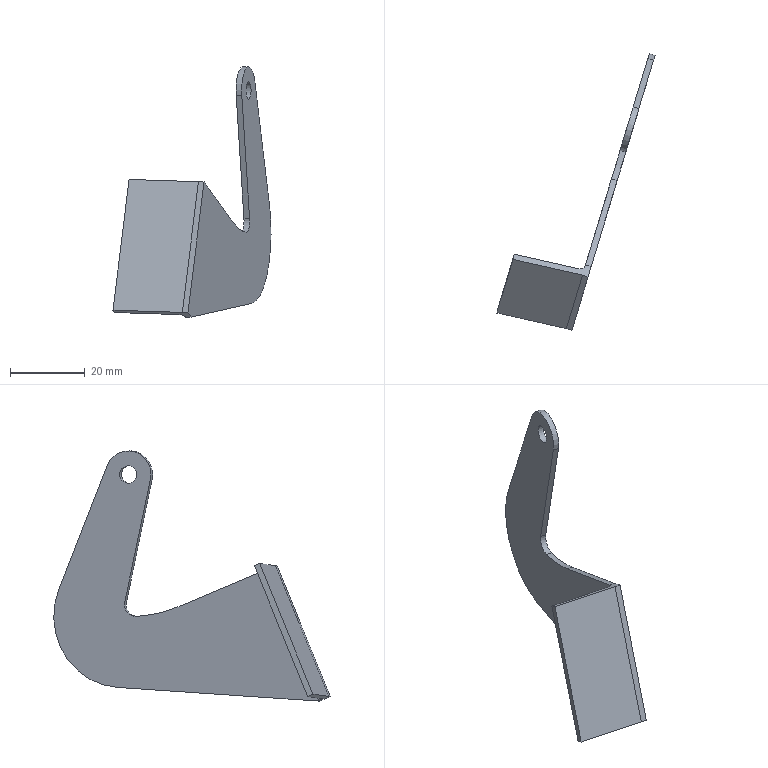Part | NX | features NG well(left door) 2 | 1 solid | 18 faces | box 42.372 x 74.153 x 67.068 mm | volume 4886 mm3 | plane 12 | cylinder 6 | commonest cylinder face diameters 3.15 x1 4.763 x1 6.35 x1 12.7 x1 38.1 x1 76.2 x1
STEP:
#1=CARTESIAN_POINT('',(564.181,-448.408,122.365));
#2=VERTEX_POINT('',#1);
#3=CARTESIAN_POINT('',(563.493,-450.688,122.365));
#4=DIRECTION('',(0.9572,-0.2893,0.));
#5=DIRECTION('',(0.2893,0.9572,0.));
#6=AXIS2_PLACEMENT_3D('',#3,#4,#5);
#7=CIRCLE('',#6,2.381);
#8=EDGE_CURVE('',#2,#2,#7,.T.);
#9=ORIENTED_EDGE('',*,*,#8,.T.);
#10=EDGE_LOOP('',(#9));
#11=FACE_BOUND('',#10,.T.);
#12=CARTESIAN_POINT('',(548.067,-501.732,61.701));
#13=VERTEX_POINT('',#12);
#14=CARTESIAN_POINT('',(548.105,-501.609,61.647));
#15=VERTEX_POINT('',#14);
#16=CARTESIAN_POINT('',(548.105,-501.609,61.647));
#17=DIRECTION('',(0.2662,0.8808,-0.3916));
#18=VECTOR('',#17,1000.);
#19=LINE('',#16,#18);
#20=EDGE_CURVE('',#13,#15,#19,.T.);
#21=ORIENTED_EDGE('',*,*,#20,.F.);
#22=CARTESIAN_POINT('',(552.384,-487.448,96.758));
#23=VERTEX_POINT('',#22);
#24=CARTESIAN_POINT('',(552.384,-487.448,96.758));
#25=DIRECTION('',(-0.1133,-0.3749,-0.9201));
#26=VECTOR('',#25,1000.);
#27=LINE('',#24,#26);
#28=EDGE_CURVE('',#13,#23,#27,.F.);
#29=ORIENTED_EDGE('',*,*,#28,.T.);
#30=CARTESIAN_POINT('',(552.421,-487.325,96.703));
#31=VERTEX_POINT('',#30);
#32=CARTESIAN_POINT('',(551.576,-490.122,97.947));
#33=DIRECTION('',(-0.2662,-0.8808,0.3916));
#34=VECTOR('',#33,1000.);
#35=LINE('',#32,#34);
#36=EDGE_CURVE('',#31,#23,#35,.T.);
#37=ORIENTED_EDGE('',*,*,#36,.F.);
#38=CARTESIAN_POINT('',(559.376,-464.31,87.022));
#39=VERTEX_POINT('',#38);
#40=CARTESIAN_POINT('',(552.421,-487.325,96.703));
#41=DIRECTION('',(-0.2683,-0.888,0.3735));
#42=VECTOR('',#41,1000.);
#43=LINE('',#40,#42);
#44=EDGE_CURVE('',#39,#31,#43,.T.);
#45=ORIENTED_EDGE('',*,*,#44,.F.);
#46=CARTESIAN_POINT('',(562.822,-452.908,84.336));
#47=VERTEX_POINT('',#46);
#48=CARTESIAN_POINT('',(563.493,-450.688,122.365));
#49=DIRECTION('',(-0.9572,0.2893,0.));
#50=DIRECTION('',(0.2893,0.9572,0.));
#51=AXIS2_PLACEMENT_3D('',#48,#49,#50);
#52=CIRCLE('',#51,38.1);
#53=EDGE_CURVE('',#47,#39,#52,.T.);
#54=ORIENTED_EDGE('',*,*,#53,.F.);
#55=CARTESIAN_POINT('',(563.775,-449.754,88.183));
#56=VERTEX_POINT('',#55);
#57=CARTESIAN_POINT('',(562.877,-452.723,87.505));
#58=DIRECTION('',(0.9572,-0.2893,0.));
#59=DIRECTION('',(0.2893,0.9572,0.));
#60=AXIS2_PLACEMENT_3D('',#57,#58,#59);
#61=CIRCLE('',#60,3.175);
#62=EDGE_CURVE('',#47,#56,#61,.T.);
#63=ORIENTED_EDGE('',*,*,#62,.T.);
#64=CARTESIAN_POINT('',(561.698,-456.626,121.008));
#65=VERTEX_POINT('',#64);
#66=CARTESIAN_POINT('',(561.698,-456.626,121.008));
#67=DIRECTION('',(0.0618,0.2045,-0.9769));
#68=VECTOR('',#67,1000.);
#69=LINE('',#66,#68);
#70=EDGE_CURVE('',#65,#56,#69,.T.);
#71=ORIENTED_EDGE('',*,*,#70,.F.);
#72=CARTESIAN_POINT('',(565.193,-445.06,124.766));
#73=VERTEX_POINT('',#72);
#74=CARTESIAN_POINT('',(563.493,-450.688,122.365));
#75=DIRECTION('',(0.9572,-0.2893,0.));
#76=DIRECTION('',(0.2893,0.9572,0.));
#77=AXIS2_PLACEMENT_3D('',#74,#75,#76);
#78=CIRCLE('',#77,6.35);
#79=EDGE_CURVE('',#73,#65,#78,.T.);
#80=ORIENTED_EDGE('',*,*,#79,.F.);
#81=CARTESIAN_POINT('',(569.121,-432.061,91.511));
#82=VERTEX_POINT('',#81);
#83=CARTESIAN_POINT('',(565.193,-445.06,124.766));
#84=DIRECTION('',(-0.1094,-0.3619,0.9258));
#85=VECTOR('',#84,1000.);
#86=LINE('',#83,#85);
#87=EDGE_CURVE('',#82,#73,#86,.T.);
#88=ORIENTED_EDGE('',*,*,#87,.F.);
#89=CARTESIAN_POINT('',(564.377,-447.762,65.299));
#90=VERTEX_POINT('',#89);
#91=CARTESIAN_POINT('',(564.02,-448.943,84.309));
#92=DIRECTION('',(0.9572,-0.2893,0.));
#93=DIRECTION('',(0.2893,0.9572,0.));
#94=AXIS2_PLACEMENT_3D('',#91,#92,#93);
#95=CIRCLE('',#94,19.05);
#96=EDGE_CURVE('',#90,#82,#95,.T.);
#97=ORIENTED_EDGE('',*,*,#96,.F.);
#98=CARTESIAN_POINT('',(548.105,-501.609,61.647));
#99=DIRECTION('',(0.2887,0.9552,0.06478));
#100=VECTOR('',#99,1000.);
#101=LINE('',#98,#100);
#102=EDGE_CURVE('',#15,#90,#101,.T.);
#103=ORIENTED_EDGE('',*,*,#102,.F.);
#104=EDGE_LOOP('',(#21,#29,#37,#45,#54,#63,#71,#80,#88,#97,#103));
#105=FACE_BOUND('',#104,.T.);
#106=CARTESIAN_POINT('',(563.493,-450.688,122.365));
#107=DIRECTION('',(0.9572,-0.2893,0.));
#108=DIRECTION('',(0.2893,0.9572,0.));
#109=AXIS2_PLACEMENT_3D('',#106,#107,#108);
#110=PLANE('',#109);
#111=ADVANCED_FACE('',(#11,#105),#110,.F.);
#112=ORIENTED_EDGE('',*,*,#36,.T.);
#113=CARTESIAN_POINT('',(550.577,-488.411,97.373));
#114=VERTEX_POINT('',#113);
#115=CARTESIAN_POINT('',(550.876,-486.992,96.758));
#116=DIRECTION('',(0.1133,0.3749,0.9201));
#117=DIRECTION('',(0.,-0.9261,0.3773));
#118=AXIS2_PLACEMENT_3D('',#115,#116,#117);
#119=CIRCLE('',#118,1.575);
#120=EDGE_CURVE('',#23,#114,#119,.F.);
#121=ORIENTED_EDGE('',*,*,#120,.T.);
#122=CARTESIAN_POINT('',(533.282,-484.519,97.916));
#123=VERTEX_POINT('',#122);
#124=CARTESIAN_POINT('',(553.407,-489.048,97.284));
#125=DIRECTION('',(0.9751,-0.2195,-0.03065));
#126=VECTOR('',#125,1000.);
#127=LINE('',#124,#126);
#128=EDGE_CURVE('',#123,#114,#127,.T.);
#129=ORIENTED_EDGE('',*,*,#128,.F.);
#130=CARTESIAN_POINT('',(532.982,-485.937,98.531));
#131=VERTEX_POINT('',#130);
#132=CARTESIAN_POINT('',(533.282,-484.519,97.916));
#133=DIRECTION('',(-0.1904,-0.9007,0.3904));
#134=VECTOR('',#133,1000.);
#135=LINE('',#132,#134);
#136=EDGE_CURVE('',#123,#131,#135,.T.);
#137=ORIENTED_EDGE('',*,*,#136,.T.);
#138=CARTESIAN_POINT('',(551.576,-490.122,97.947));
#139=VERTEX_POINT('',#138);
#140=CARTESIAN_POINT('',(553.107,-490.466,97.899));
#141=DIRECTION('',(0.9751,-0.2195,-0.03065));
#142=VECTOR('',#141,1000.);
#143=LINE('',#140,#142);
#144=EDGE_CURVE('',#131,#139,#143,.T.);
#145=ORIENTED_EDGE('',*,*,#144,.T.);
#146=CARTESIAN_POINT('',(553.083,-490.577,97.947));
#147=VERTEX_POINT('',#146);
#148=CARTESIAN_POINT('',(551.576,-490.122,97.947));
#149=DIRECTION('',(0.9572,-0.2893,0.));
#150=VECTOR('',#149,1000.);
#151=LINE('',#148,#150);
#152=EDGE_CURVE('',#139,#147,#151,.T.);
#153=ORIENTED_EDGE('',*,*,#152,.T.);
#154=CARTESIAN_POINT('',(553.928,-487.781,96.703));
#155=VERTEX_POINT('',#154);
#156=CARTESIAN_POINT('',(553.083,-490.577,97.947));
#157=DIRECTION('',(-0.2662,-0.8808,0.3916));
#158=VECTOR('',#157,1000.);
#159=LINE('',#156,#158);
#160=EDGE_CURVE('',#155,#147,#159,.T.);
#161=ORIENTED_EDGE('',*,*,#160,.F.);
#162=CARTESIAN_POINT('',(552.421,-487.325,96.703));
#163=DIRECTION('',(0.9572,-0.2893,0.));
#164=VECTOR('',#163,1000.);
#165=LINE('',#162,#164);
#166=EDGE_CURVE('',#31,#155,#165,.T.);
#167=ORIENTED_EDGE('',*,*,#166,.F.);
#168=EDGE_LOOP('',(#112,#121,#129,#137,#145,#153,#161,#167));
#169=FACE_BOUND('',#168,.T.);
#170=CARTESIAN_POINT('',(551.576,-490.122,97.947));
#171=DIRECTION('',(0.1133,0.3749,0.9201));
#172=DIRECTION('',(0.,-0.9261,0.3773));
#173=AXIS2_PLACEMENT_3D('',#170,#171,#172);
#174=PLANE('',#173);
#175=ADVANCED_FACE('',(#169),#174,.T.);
#176=CARTESIAN_POINT('',(560.883,-464.766,87.022));
#177=VERTEX_POINT('',#176);
#178=CARTESIAN_POINT('',(553.928,-487.781,96.703));
#179=DIRECTION('',(-0.2683,-0.888,0.3735));
#180=VECTOR('',#179,1000.);
#181=LINE('',#178,#180);
#182=EDGE_CURVE('',#177,#155,#181,.T.);
#183=ORIENTED_EDGE('',*,*,#182,.F.);
#184=CARTESIAN_POINT('',(559.376,-464.31,87.022));
#185=DIRECTION('',(0.9572,-0.2893,0.));
#186=VECTOR('',#185,1000.);
#187=LINE('',#184,#186);
#188=EDGE_CURVE('',#39,#177,#187,.T.);
#189=ORIENTED_EDGE('',*,*,#188,.F.);
#190=ORIENTED_EDGE('',*,*,#44,.T.);
#191=ORIENTED_EDGE('',*,*,#166,.T.);
#192=EDGE_LOOP('',(#183,#189,#190,#191));
#193=FACE_BOUND('',#192,.T.);
#194=CARTESIAN_POINT('',(552.421,-487.325,96.703));
#195=DIRECTION('',(0.108,0.3575,0.9276));
#196=DIRECTION('',(0.,-0.9331,0.3596));
#197=AXIS2_PLACEMENT_3D('',#194,#195,#196);
#198=PLANE('',#197);
#199=ADVANCED_FACE('',(#193),#198,.T.);
#200=CARTESIAN_POINT('',(564.329,-453.364,84.336));
#201=VERTEX_POINT('',#200);
#202=CARTESIAN_POINT('',(565.,-451.143,122.365));
#203=DIRECTION('',(-0.9572,0.2893,0.));
#204=DIRECTION('',(0.2893,0.9572,0.));
#205=AXIS2_PLACEMENT_3D('',#202,#203,#204);
#206=CIRCLE('',#205,38.1);
#207=EDGE_CURVE('',#201,#177,#206,.T.);
#208=ORIENTED_EDGE('',*,*,#207,.F.);
#209=CARTESIAN_POINT('',(562.822,-452.908,84.336));
#210=DIRECTION('',(0.9572,-0.2893,0.));
#211=VECTOR('',#210,1000.);
#212=LINE('',#209,#211);
#213=EDGE_CURVE('',#201,#47,#212,.F.);
#214=ORIENTED_EDGE('',*,*,#213,.T.);
#215=ORIENTED_EDGE('',*,*,#53,.T.);
#216=ORIENTED_EDGE('',*,*,#188,.T.);
#217=EDGE_LOOP('',(#208,#214,#215,#216));
#218=FACE_BOUND('',#217,.T.);
#219=CARTESIAN_POINT('',(563.493,-450.688,122.365));
#220=DIRECTION('',(0.9572,-0.2893,0.));
#221=DIRECTION('',(0.2893,0.9572,0.));
#222=AXIS2_PLACEMENT_3D('',#219,#220,#221);
#223=CYLINDRICAL_SURFACE('',#222,38.1);
#224=ADVANCED_FACE('',(#218),#223,.F.);
#225=ORIENTED_EDGE('',*,*,#70,.T.);
#226=CARTESIAN_POINT('',(565.282,-450.21,88.183));
#227=VERTEX_POINT('',#226);
#228=CARTESIAN_POINT('',(565.282,-450.21,88.183));
#229=DIRECTION('',(-0.9572,0.2893,0.));
#230=VECTOR('',#229,1000.);
#231=LINE('',#228,#230);
#232=EDGE_CURVE('',#56,#227,#231,.F.);
#233=ORIENTED_EDGE('',*,*,#232,.T.);
#234=CARTESIAN_POINT('',(563.206,-457.082,121.008));
#235=VERTEX_POINT('',#234);
#236=CARTESIAN_POINT('',(563.206,-457.082,121.008));
#237=DIRECTION('',(0.0618,0.2045,-0.9769));
#238=VECTOR('',#237,1000.);
#239=LINE('',#236,#238);
#240=EDGE_CURVE('',#235,#227,#239,.T.);
#241=ORIENTED_EDGE('',*,*,#240,.F.);
#242=CARTESIAN_POINT('',(561.698,-456.626,121.008));
#243=DIRECTION('',(0.9572,-0.2893,0.));
#244=VECTOR('',#243,1000.);
#245=LINE('',#242,#244);
#246=EDGE_CURVE('',#65,#235,#245,.T.);
#247=ORIENTED_EDGE('',*,*,#246,.F.);
#248=EDGE_LOOP('',(#225,#233,#241,#247));
#249=FACE_BOUND('',#248,.T.);
#250=CARTESIAN_POINT('',(561.698,-456.626,121.008));
#251=DIRECTION('',(-0.2826,-0.9351,-0.2136));
#252=DIRECTION('',(0.9572,-0.2893,0.));
#253=AXIS2_PLACEMENT_3D('',#250,#251,#252);
#254=PLANE('',#253);
#255=ADVANCED_FACE('',(#249),#254,.T.);
#256=CARTESIAN_POINT('',(566.701,-445.516,124.766));
#257=VERTEX_POINT('',#256);
#258=CARTESIAN_POINT('',(565.,-451.143,122.365));
#259=DIRECTION('',(0.9572,-0.2893,0.));
#260=DIRECTION('',(0.2893,0.9572,0.));
#261=AXIS2_PLACEMENT_3D('',#258,#259,#260);
#262=CIRCLE('',#261,6.35);
#263=EDGE_CURVE('',#257,#235,#262,.T.);
#264=ORIENTED_EDGE('',*,*,#263,.F.);
#265=CARTESIAN_POINT('',(565.193,-445.06,124.766));
#266=DIRECTION('',(0.9572,-0.2893,0.));
#267=VECTOR('',#266,1000.);
#268=LINE('',#265,#267);
#269=EDGE_CURVE('',#73,#257,#268,.T.);
#270=ORIENTED_EDGE('',*,*,#269,.F.);
#271=ORIENTED_EDGE('',*,*,#79,.T.);
#272=ORIENTED_EDGE('',*,*,#246,.T.);
#273=EDGE_LOOP('',(#264,#270,#271,#272));
#274=FACE_BOUND('',#273,.T.);
#275=CARTESIAN_POINT('',(563.493,-450.688,122.365));
#276=DIRECTION('',(0.9572,-0.2893,0.));
#277=DIRECTION('',(0.2893,0.9572,0.));
#278=AXIS2_PLACEMENT_3D('',#275,#276,#277);
#279=CYLINDRICAL_SURFACE('',#278,6.35);
#280=ADVANCED_FACE('',(#274),#279,.T.);
#281=CARTESIAN_POINT('',(570.629,-432.516,91.511));
#282=VERTEX_POINT('',#281);
#283=CARTESIAN_POINT('',(566.701,-445.516,124.766));
#284=DIRECTION('',(-0.1094,-0.3619,0.9258));
#285=VECTOR('',#284,1000.);
#286=LINE('',#283,#285);
#287=EDGE_CURVE('',#282,#257,#286,.T.);
#288=ORIENTED_EDGE('',*,*,#287,.F.);
#289=CARTESIAN_POINT('',(569.121,-432.061,91.511));
#290=DIRECTION('',(0.9572,-0.2893,0.));
#291=VECTOR('',#290,1000.);
#292=LINE('',#289,#291);
#293=EDGE_CURVE('',#82,#282,#292,.T.);
#294=ORIENTED_EDGE('',*,*,#293,.F.);
#295=ORIENTED_EDGE('',*,*,#87,.T.);
#296=ORIENTED_EDGE('',*,*,#269,.T.);
#297=EDGE_LOOP('',(#288,#294,#295,#296));
#298=FACE_BOUND('',#297,.T.);
#299=CARTESIAN_POINT('',(565.193,-445.06,124.766));
#300=DIRECTION('',(0.2678,0.8862,0.3781));
#301=DIRECTION('',(0.,-0.3924,0.9198));
#302=AXIS2_PLACEMENT_3D('',#299,#300,#301);
#303=PLANE('',#302);
#304=ADVANCED_FACE('',(#298),#303,.T.);
#305=CARTESIAN_POINT('',(565.884,-448.217,65.299));
#306=VERTEX_POINT('',#305);
#307=CARTESIAN_POINT('',(565.527,-449.399,84.309));
#308=DIRECTION('',(0.9572,-0.2893,0.));
#309=DIRECTION('',(0.2893,0.9572,0.));
#310=AXIS2_PLACEMENT_3D('',#307,#308,#309);
#311=CIRCLE('',#310,19.05);
#312=EDGE_CURVE('',#306,#282,#311,.T.);
#313=ORIENTED_EDGE('',*,*,#312,.F.);
#314=CARTESIAN_POINT('',(564.377,-447.762,65.299));
#315=DIRECTION('',(0.9572,-0.2893,0.));
#316=VECTOR('',#315,1000.);
#317=LINE('',#314,#316);
#318=EDGE_CURVE('',#90,#306,#317,.T.);
#319=ORIENTED_EDGE('',*,*,#318,.F.);
#320=ORIENTED_EDGE('',*,*,#96,.T.);
#321=ORIENTED_EDGE('',*,*,#293,.T.);
#322=EDGE_LOOP('',(#313,#319,#320,#321));
#323=FACE_BOUND('',#322,.T.);
#324=CARTESIAN_POINT('',(564.02,-448.943,84.309));
#325=DIRECTION('',(0.9572,-0.2893,0.));
#326=DIRECTION('',(0.2893,0.9572,0.));
#327=AXIS2_PLACEMENT_3D('',#324,#325,#326);
#328=CYLINDRICAL_SURFACE('',#327,19.05);
#329=ADVANCED_FACE('',(#323),#328,.T.);
#330=CARTESIAN_POINT('',(549.612,-502.064,61.647));
#331=VERTEX_POINT('',#330);
#332=CARTESIAN_POINT('',(549.612,-502.064,61.647));
#333=DIRECTION('',(0.2887,0.9552,0.06478));
#334=VECTOR('',#333,1000.);
#335=LINE('',#332,#334);
#336=EDGE_CURVE('',#331,#306,#335,.T.);
#337=ORIENTED_EDGE('',*,*,#336,.F.);
#338=CARTESIAN_POINT('',(548.105,-501.609,61.647));
#339=DIRECTION('',(0.9572,-0.2893,0.));
#340=VECTOR('',#339,1000.);
#341=LINE('',#338,#340);
#342=EDGE_CURVE('',#15,#331,#341,.T.);
#343=ORIENTED_EDGE('',*,*,#342,.F.);
#344=ORIENTED_EDGE('',*,*,#102,.T.);
#345=ORIENTED_EDGE('',*,*,#318,.T.);
#346=EDGE_LOOP('',(#337,#343,#344,#345));
#347=FACE_BOUND('',#346,.T.);
#348=CARTESIAN_POINT('',(548.105,-501.609,61.647));
#349=DIRECTION('',(0.01874,0.06201,-0.9979));
#350=DIRECTION('',(0.,0.9981,0.06202));
#351=AXIS2_PLACEMENT_3D('',#348,#349,#350);
#352=PLANE('',#351);
#353=ADVANCED_FACE('',(#347),#352,.T.);
#354=CARTESIAN_POINT('',(546.26,-502.694,62.316));
#355=VERTEX_POINT('',#354);
#356=CARTESIAN_POINT('',(528.966,-498.802,62.86));
#357=VERTEX_POINT('',#356);
#358=CARTESIAN_POINT('',(528.966,-498.802,62.86));
#359=DIRECTION('',(-0.9751,0.2195,0.03065));
#360=VECTOR('',#359,1000.);
#361=LINE('',#358,#360);
#362=EDGE_CURVE('',#355,#357,#361,.T.);
#363=ORIENTED_EDGE('',*,*,#362,.F.);
#364=CARTESIAN_POINT('',(546.56,-501.276,61.701));
#365=DIRECTION('',(-0.1133,-0.3749,-0.9201));
#366=DIRECTION('',(0.,0.9261,-0.3773));
#367=AXIS2_PLACEMENT_3D('',#364,#365,#366);
#368=CIRCLE('',#367,1.575);
#369=EDGE_CURVE('',#355,#13,#368,.F.);
#370=ORIENTED_EDGE('',*,*,#369,.T.);
#371=ORIENTED_EDGE('',*,*,#20,.T.);
#372=ORIENTED_EDGE('',*,*,#342,.T.);
#373=CARTESIAN_POINT('',(548.767,-504.861,62.89));
#374=VERTEX_POINT('',#373);
#375=CARTESIAN_POINT('',(549.612,-502.064,61.647));
#376=DIRECTION('',(0.2662,0.8808,-0.3916));
#377=VECTOR('',#376,1000.);
#378=LINE('',#375,#377);
#379=EDGE_CURVE('',#374,#331,#378,.T.);
#380=ORIENTED_EDGE('',*,*,#379,.F.);
#381=CARTESIAN_POINT('',(547.259,-504.405,62.89));
#382=VERTEX_POINT('',#381);
#383=CARTESIAN_POINT('',(547.259,-504.405,62.89));
#384=DIRECTION('',(0.9572,-0.2893,0.));
#385=VECTOR('',#384,1000.);
#386=LINE('',#383,#385);
#387=EDGE_CURVE('',#382,#374,#386,.T.);
#388=ORIENTED_EDGE('',*,*,#387,.F.);
#389=CARTESIAN_POINT('',(528.666,-500.221,63.475));
#390=VERTEX_POINT('',#389);
#391=CARTESIAN_POINT('',(528.666,-500.221,63.475));
#392=DIRECTION('',(-0.9751,0.2195,0.03065));
#393=VECTOR('',#392,1000.);
#394=LINE('',#391,#393);
#395=EDGE_CURVE('',#382,#390,#394,.T.);
#396=ORIENTED_EDGE('',*,*,#395,.T.);
#397=CARTESIAN_POINT('',(528.966,-498.802,62.86));
#398=DIRECTION('',(-0.1904,-0.9007,0.3904));
#399=VECTOR('',#398,1000.);
#400=LINE('',#397,#399);
#401=EDGE_CURVE('',#357,#390,#400,.T.);
#402=ORIENTED_EDGE('',*,*,#401,.F.);
#403=EDGE_LOOP('',(#363,#370,#371,#372,#380,#388,#396,#402));
#404=FACE_BOUND('',#403,.T.);
#405=CARTESIAN_POINT('',(548.105,-501.609,61.647));
#406=DIRECTION('',(-0.1133,-0.3749,-0.9201));
#407=DIRECTION('',(0.,0.9261,-0.3773));
#408=AXIS2_PLACEMENT_3D('',#405,#406,#407);
#409=PLANE('',#408);
#410=ADVANCED_FACE('',(#404),#409,.T.);
#411=CARTESIAN_POINT('',(553.083,-490.577,97.947));
#412=DIRECTION('',(-0.1133,-0.3749,-0.9201));
#413=VECTOR('',#412,1000.);
#414=LINE('',#411,#413);
#415=EDGE_CURVE('',#147,#374,#414,.T.);
#416=ORIENTED_EDGE('',*,*,#415,.F.);
#417=ORIENTED_EDGE('',*,*,#152,.F.);
#418=CARTESIAN_POINT('',(551.576,-490.122,97.947));
#419=DIRECTION('',(-0.1133,-0.3749,-0.9201));
#420=VECTOR('',#419,1000.);
#421=LINE('',#418,#420);
#422=EDGE_CURVE('',#139,#382,#421,.T.);
#423=ORIENTED_EDGE('',*,*,#422,.T.);
#424=ORIENTED_EDGE('',*,*,#387,.T.);
#425=EDGE_LOOP('',(#416,#417,#423,#424));
#426=FACE_BOUND('',#425,.T.);
#427=CARTESIAN_POINT('',(551.576,-490.122,97.947));
#428=DIRECTION('',(-0.2662,-0.8808,0.3916));
#429=DIRECTION('',(0.,-0.4063,-0.9137));
#430=AXIS2_PLACEMENT_3D('',#427,#428,#429);
#431=PLANE('',#430);
#432=ADVANCED_FACE('',(#426),#431,.T.);
#433=CARTESIAN_POINT('',(565.689,-448.864,122.365));
#434=VERTEX_POINT('',#433);
#435=CARTESIAN_POINT('',(565.,-451.143,122.365));
#436=DIRECTION('',(0.9572,-0.2893,0.));
#437=DIRECTION('',(0.2893,0.9572,0.));
#438=AXIS2_PLACEMENT_3D('',#435,#436,#437);
#439=CIRCLE('',#438,2.381);
#440=EDGE_CURVE('',#434,#434,#439,.T.);
#441=ORIENTED_EDGE('',*,*,#440,.F.);
#442=EDGE_LOOP('',(#441));
#443=FACE_BOUND('',#442,.T.);
#444=ORIENTED_EDGE('',*,*,#160,.T.);
#445=ORIENTED_EDGE('',*,*,#415,.T.);
#446=ORIENTED_EDGE('',*,*,#379,.T.);
#447=ORIENTED_EDGE('',*,*,#336,.T.);
#448=ORIENTED_EDGE('',*,*,#312,.T.);
#449=ORIENTED_EDGE('',*,*,#287,.T.);
#450=ORIENTED_EDGE('',*,*,#263,.T.);
#451=ORIENTED_EDGE('',*,*,#240,.T.);
#452=CARTESIAN_POINT('',(564.385,-453.179,87.505));
#453=DIRECTION('',(0.9572,-0.2893,0.));
#454=DIRECTION('',(0.2893,0.9572,0.));
#455=AXIS2_PLACEMENT_3D('',#452,#453,#454);
#456=CIRCLE('',#455,3.175);
#457=EDGE_CURVE('',#227,#201,#456,.F.);
#458=ORIENTED_EDGE('',*,*,#457,.T.);
#459=ORIENTED_EDGE('',*,*,#207,.T.);
#460=ORIENTED_EDGE('',*,*,#182,.T.);
#461=EDGE_LOOP('',(#444,#445,#446,#447,#448,#449,#450,#451,#458,#459,#460));
#462=FACE_BOUND('',#461,.T.);
#463=CARTESIAN_POINT('',(565.,-451.143,122.365));
#464=DIRECTION('',(0.9572,-0.2893,0.));
#465=DIRECTION('',(0.2893,0.9572,0.));
#466=AXIS2_PLACEMENT_3D('',#463,#464,#465);
#467=PLANE('',#466);
#468=ADVANCED_FACE('',(#443,#462),#467,.T.);
#469=ORIENTED_EDGE('',*,*,#8,.F.);
#470=EDGE_LOOP('',(#469));
#471=FACE_BOUND('',#470,.T.);
#472=ORIENTED_EDGE('',*,*,#440,.T.);
#473=EDGE_LOOP('',(#472));
#474=FACE_BOUND('',#473,.T.);
#475=CARTESIAN_POINT('',(563.493,-450.688,122.365));
#476=DIRECTION('',(0.9572,-0.2893,0.));
#477=DIRECTION('',(0.2893,0.9572,0.));
#478=AXIS2_PLACEMENT_3D('',#475,#476,#477);
#479=CYLINDRICAL_SURFACE('',#478,2.381);
#480=ADVANCED_FACE('',(#471,#474),#479,.F.);
#481=ORIENTED_EDGE('',*,*,#62,.F.);
#482=ORIENTED_EDGE('',*,*,#213,.F.);
#483=ORIENTED_EDGE('',*,*,#457,.F.);
#484=ORIENTED_EDGE('',*,*,#232,.F.);
#485=EDGE_LOOP('',(#481,#482,#483,#484));
#486=FACE_BOUND('',#485,.T.);
#487=CARTESIAN_POINT('',(562.877,-452.723,87.505));
#488=DIRECTION('',(0.9572,-0.2893,0.));
#489=DIRECTION('',(0.2893,0.9572,0.));
#490=AXIS2_PLACEMENT_3D('',#487,#488,#489);
#491=CYLINDRICAL_SURFACE('',#490,3.175);
#492=ADVANCED_FACE('',(#486),#491,.F.);
#493=ORIENTED_EDGE('',*,*,#128,.T.);
#494=CARTESIAN_POINT('',(546.26,-502.694,62.316));
#495=DIRECTION('',(-0.1133,-0.3749,-0.9201));
#496=VECTOR('',#495,1000.);
#497=LINE('',#494,#496);
#498=EDGE_CURVE('',#114,#355,#497,.T.);
#499=ORIENTED_EDGE('',*,*,#498,.T.);
#500=ORIENTED_EDGE('',*,*,#362,.T.);
#501=CARTESIAN_POINT('',(533.282,-484.519,97.916));
#502=DIRECTION('',(0.1133,0.3749,0.9201));
#503=VECTOR('',#502,1000.);
#504=LINE('',#501,#503);
#505=EDGE_CURVE('',#357,#123,#504,.T.);
#506=ORIENTED_EDGE('',*,*,#505,.T.);
#507=EDGE_LOOP('',(#493,#499,#500,#506));
#508=FACE_BOUND('',#507,.T.);
#509=CARTESIAN_POINT('',(549.09,-503.331,62.227));
#510=DIRECTION('',(-0.1904,-0.9007,0.3904));
#511=DIRECTION('',(0.,-0.3977,-0.9175));
#512=AXIS2_PLACEMENT_3D('',#509,#510,#511);
#513=PLANE('',#512);
#514=ADVANCED_FACE('',(#508),#513,.F.);
#515=ORIENTED_EDGE('',*,*,#422,.F.);
#516=ORIENTED_EDGE('',*,*,#144,.F.);
#517=CARTESIAN_POINT('',(532.982,-485.937,98.531));
#518=DIRECTION('',(0.1133,0.3749,0.9201));
#519=VECTOR('',#518,1000.);
#520=LINE('',#517,#519);
#521=EDGE_CURVE('',#390,#131,#520,.T.);
#522=ORIENTED_EDGE('',*,*,#521,.F.);
#523=ORIENTED_EDGE('',*,*,#395,.F.);
#524=EDGE_LOOP('',(#515,#516,#522,#523));
#525=FACE_BOUND('',#524,.T.);
#526=CARTESIAN_POINT('',(548.79,-504.75,62.842));
#527=DIRECTION('',(-0.1904,-0.9007,0.3904));
#528=DIRECTION('',(0.,-0.3977,-0.9175));
#529=AXIS2_PLACEMENT_3D('',#526,#527,#528);
#530=PLANE('',#529);
#531=ADVANCED_FACE('',(#525),#530,.T.);
#532=ORIENTED_EDGE('',*,*,#521,.T.);
#533=ORIENTED_EDGE('',*,*,#136,.F.);
#534=ORIENTED_EDGE('',*,*,#505,.F.);
#535=ORIENTED_EDGE('',*,*,#401,.T.);
#536=EDGE_LOOP('',(#532,#533,#534,#535));
#537=FACE_BOUND('',#536,.T.);
#538=CARTESIAN_POINT('',(533.282,-484.519,97.916));
#539=DIRECTION('',(0.9751,-0.2195,-0.03065));
#540=DIRECTION('',(0.2196,0.9756,0.));
#541=AXIS2_PLACEMENT_3D('',#538,#539,#540);
#542=PLANE('',#541);
#543=ADVANCED_FACE('',(#537),#542,.F.);
#544=ORIENTED_EDGE('',*,*,#120,.F.);
#545=ORIENTED_EDGE('',*,*,#28,.F.);
#546=ORIENTED_EDGE('',*,*,#369,.F.);
#547=ORIENTED_EDGE('',*,*,#498,.F.);
#548=EDGE_LOOP('',(#544,#545,#546,#547));
#549=FACE_BOUND('',#548,.T.);
#550=CARTESIAN_POINT('',(546.56,-501.276,61.701));
#551=DIRECTION('',(0.1133,0.3749,0.9201));
#552=DIRECTION('',(0.,-0.9261,0.3773));
#553=AXIS2_PLACEMENT_3D('',#550,#551,#552);
#554=CYLINDRICAL_SURFACE('',#553,1.575);
#555=ADVANCED_FACE('',(#549),#554,.F.);
#556=CLOSED_SHELL('',(#111,#175,#199,#224,#255,#280,#304,#329,#353,#410,#432,#468,#480,#492,#514,#531,#543,#555));
#557=MANIFOLD_SOLID_BREP('',#556);
#558=(LENGTH_UNIT()NAMED_UNIT(*)SI_UNIT(.MILLI.,.METRE.));
#559=UNCERTAINTY_MEASURE_WITH_UNIT(LENGTH_MEASURE(0.00001),#558,'','');
#560=(NAMED_UNIT(*)PLANE_ANGLE_UNIT()SI_UNIT($,.RADIAN.));
#561=(NAMED_UNIT(*)SI_UNIT($,.STERADIAN.)SOLID_ANGLE_UNIT());
#562=(GEOMETRIC_REPRESENTATION_CONTEXT(3)GLOBAL_UNCERTAINTY_ASSIGNED_CONTEXT((#559))GLOBAL_UNIT_ASSIGNED_CONTEXT((#558,#560,#561))REPRESENTATION_CONTEXT('',''));
#563=ADVANCED_BREP_SHAPE_REPRESENTATION('',(#557),#562);